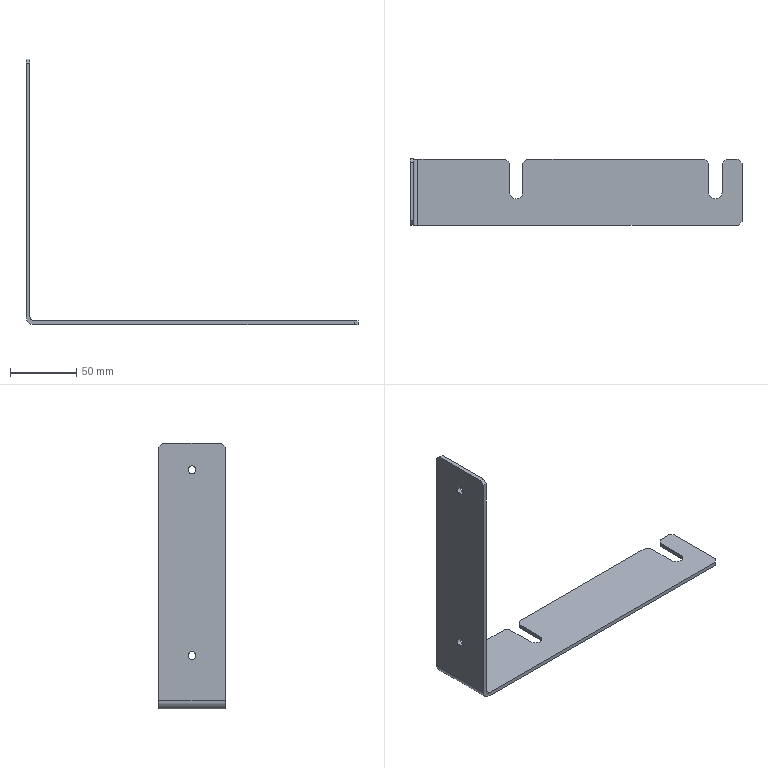Part | STEP file | J452-EBZ05-28-08-Part-2 | 1 solid | 30 faces | box 250 x 50 x 200 mm | volume 64747 mm3 | plane 22 | cylinder 8 | commonest cylinder face diameters 6 x5 10 x2 12 x1